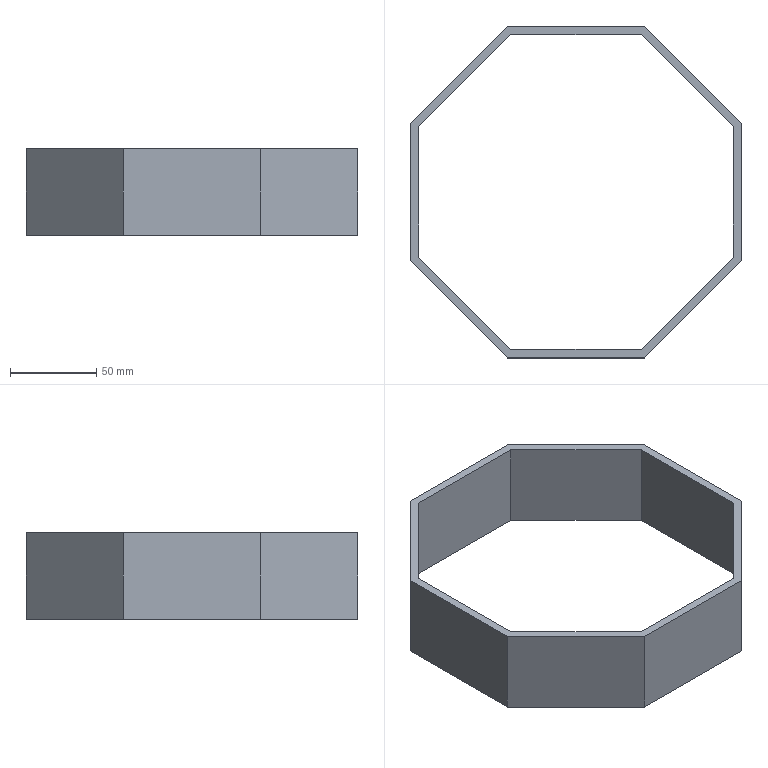Part | SolidWorks | features Extrusion 1, ICE 1 | 1 solid | 18 faces | box 192.167 x 192.167 x 50 mm | volume 155054 mm3 | plane 18
STEP:
#1=CARTESIAN_POINT('',(39.799,96.083,0.));
#2=VERTEX_POINT('',#1);
#3=CARTESIAN_POINT('',(-39.799,96.083,0.));
#4=VERTEX_POINT('',#3);
#5=CARTESIAN_POINT('',(39.799,96.083,0.));
#6=DIRECTION('',(-1.,0.,0.));
#7=VECTOR('',#6,1000.);
#8=LINE('',#5,#7);
#9=EDGE_CURVE('',#2,#4,#8,.T.);
#10=ORIENTED_EDGE('',*,*,#9,.T.);
#11=CARTESIAN_POINT('',(-39.799,96.083,50.));
#12=VERTEX_POINT('',#11);
#13=CARTESIAN_POINT('',(-39.799,96.083,50.));
#14=DIRECTION('',(0.,0.,-1.));
#15=VECTOR('',#14,1000.);
#16=LINE('',#13,#15);
#17=EDGE_CURVE('',#12,#4,#16,.T.);
#18=ORIENTED_EDGE('',*,*,#17,.F.);
#19=CARTESIAN_POINT('',(39.799,96.083,50.));
#20=VERTEX_POINT('',#19);
#21=CARTESIAN_POINT('',(39.799,96.083,50.));
#22=DIRECTION('',(-1.,0.,0.));
#23=VECTOR('',#22,1000.);
#24=LINE('',#21,#23);
#25=EDGE_CURVE('',#20,#12,#24,.T.);
#26=ORIENTED_EDGE('',*,*,#25,.F.);
#27=CARTESIAN_POINT('',(39.799,96.083,50.));
#28=DIRECTION('',(0.,0.,-1.));
#29=VECTOR('',#28,1000.);
#30=LINE('',#27,#29);
#31=EDGE_CURVE('',#20,#2,#30,.T.);
#32=ORIENTED_EDGE('',*,*,#31,.T.);
#33=EDGE_LOOP('',(#10,#18,#26,#32));
#34=FACE_OUTER_BOUND('',#33,.T.);
#35=CARTESIAN_POINT('',(39.799,96.083,50.));
#36=DIRECTION('',(0.,-1.,0.));
#37=DIRECTION('',(0.,0.,-1.));
#38=AXIS2_PLACEMENT_3D('',#35,#36,#37);
#39=PLANE('',#38);
#40=ADVANCED_FACE('',(#34),#39,.F.);
#41=CARTESIAN_POINT('',(-96.083,39.799,0.));
#42=VERTEX_POINT('',#41);
#43=CARTESIAN_POINT('',(-39.799,96.083,0.));
#44=DIRECTION('',(-0.7071,-0.7071,0.));
#45=VECTOR('',#44,1000.);
#46=LINE('',#43,#45);
#47=EDGE_CURVE('',#4,#42,#46,.T.);
#48=ORIENTED_EDGE('',*,*,#47,.T.);
#49=CARTESIAN_POINT('',(-96.083,39.799,50.));
#50=VERTEX_POINT('',#49);
#51=CARTESIAN_POINT('',(-96.083,39.799,50.));
#52=DIRECTION('',(0.,0.,-1.));
#53=VECTOR('',#52,1000.);
#54=LINE('',#51,#53);
#55=EDGE_CURVE('',#50,#42,#54,.T.);
#56=ORIENTED_EDGE('',*,*,#55,.F.);
#57=CARTESIAN_POINT('',(-39.799,96.083,50.));
#58=DIRECTION('',(-0.7071,-0.7071,0.));
#59=VECTOR('',#58,1000.);
#60=LINE('',#57,#59);
#61=EDGE_CURVE('',#12,#50,#60,.T.);
#62=ORIENTED_EDGE('',*,*,#61,.F.);
#63=ORIENTED_EDGE('',*,*,#17,.T.);
#64=EDGE_LOOP('',(#48,#56,#62,#63));
#65=FACE_OUTER_BOUND('',#64,.T.);
#66=CARTESIAN_POINT('',(-39.799,96.083,50.));
#67=DIRECTION('',(0.7071,-0.7071,0.));
#68=DIRECTION('',(0.7071,0.7071,0.));
#69=AXIS2_PLACEMENT_3D('',#66,#67,#68);
#70=PLANE('',#69);
#71=ADVANCED_FACE('',(#65),#70,.F.);
#72=CARTESIAN_POINT('',(-96.083,-39.799,0.));
#73=VERTEX_POINT('',#72);
#74=CARTESIAN_POINT('',(-96.083,39.799,0.));
#75=DIRECTION('',(0.,-1.,0.));
#76=VECTOR('',#75,1000.);
#77=LINE('',#74,#76);
#78=EDGE_CURVE('',#42,#73,#77,.T.);
#79=ORIENTED_EDGE('',*,*,#78,.T.);
#80=CARTESIAN_POINT('',(-96.083,-39.799,50.));
#81=VERTEX_POINT('',#80);
#82=CARTESIAN_POINT('',(-96.083,-39.799,50.));
#83=DIRECTION('',(0.,0.,-1.));
#84=VECTOR('',#83,1000.);
#85=LINE('',#82,#84);
#86=EDGE_CURVE('',#81,#73,#85,.T.);
#87=ORIENTED_EDGE('',*,*,#86,.F.);
#88=CARTESIAN_POINT('',(-96.083,39.799,50.));
#89=DIRECTION('',(0.,-1.,0.));
#90=VECTOR('',#89,1000.);
#91=LINE('',#88,#90);
#92=EDGE_CURVE('',#50,#81,#91,.T.);
#93=ORIENTED_EDGE('',*,*,#92,.F.);
#94=ORIENTED_EDGE('',*,*,#55,.T.);
#95=EDGE_LOOP('',(#79,#87,#93,#94));
#96=FACE_OUTER_BOUND('',#95,.T.);
#97=CARTESIAN_POINT('',(-96.083,39.799,50.));
#98=DIRECTION('',(1.,0.,0.));
#99=DIRECTION('',(0.,1.,0.));
#100=AXIS2_PLACEMENT_3D('',#97,#98,#99);
#101=PLANE('',#100);
#102=ADVANCED_FACE('',(#96),#101,.F.);
#103=CARTESIAN_POINT('',(-39.799,-96.083,0.));
#104=VERTEX_POINT('',#103);
#105=CARTESIAN_POINT('',(-96.083,-39.799,0.));
#106=DIRECTION('',(0.7071,-0.7071,0.));
#107=VECTOR('',#106,1000.);
#108=LINE('',#105,#107);
#109=EDGE_CURVE('',#73,#104,#108,.T.);
#110=ORIENTED_EDGE('',*,*,#109,.T.);
#111=CARTESIAN_POINT('',(-39.799,-96.083,50.));
#112=VERTEX_POINT('',#111);
#113=CARTESIAN_POINT('',(-39.799,-96.083,50.));
#114=DIRECTION('',(0.,0.,-1.));
#115=VECTOR('',#114,1000.);
#116=LINE('',#113,#115);
#117=EDGE_CURVE('',#112,#104,#116,.T.);
#118=ORIENTED_EDGE('',*,*,#117,.F.);
#119=CARTESIAN_POINT('',(-96.083,-39.799,50.));
#120=DIRECTION('',(0.7071,-0.7071,0.));
#121=VECTOR('',#120,1000.);
#122=LINE('',#119,#121);
#123=EDGE_CURVE('',#81,#112,#122,.T.);
#124=ORIENTED_EDGE('',*,*,#123,.F.);
#125=ORIENTED_EDGE('',*,*,#86,.T.);
#126=EDGE_LOOP('',(#110,#118,#124,#125));
#127=FACE_OUTER_BOUND('',#126,.T.);
#128=CARTESIAN_POINT('',(-96.083,-39.799,50.));
#129=DIRECTION('',(0.7071,0.7071,0.));
#130=DIRECTION('',(-0.7071,0.7071,0.));
#131=AXIS2_PLACEMENT_3D('',#128,#129,#130);
#132=PLANE('',#131);
#133=ADVANCED_FACE('',(#127),#132,.F.);
#134=CARTESIAN_POINT('',(39.799,-96.083,0.));
#135=VERTEX_POINT('',#134);
#136=CARTESIAN_POINT('',(-39.799,-96.083,0.));
#137=DIRECTION('',(1.,0.,0.));
#138=VECTOR('',#137,1000.);
#139=LINE('',#136,#138);
#140=EDGE_CURVE('',#104,#135,#139,.T.);
#141=ORIENTED_EDGE('',*,*,#140,.T.);
#142=CARTESIAN_POINT('',(39.799,-96.083,50.));
#143=VERTEX_POINT('',#142);
#144=CARTESIAN_POINT('',(39.799,-96.083,50.));
#145=DIRECTION('',(0.,0.,-1.));
#146=VECTOR('',#145,1000.);
#147=LINE('',#144,#146);
#148=EDGE_CURVE('',#143,#135,#147,.T.);
#149=ORIENTED_EDGE('',*,*,#148,.F.);
#150=CARTESIAN_POINT('',(-39.799,-96.083,50.));
#151=DIRECTION('',(1.,0.,0.));
#152=VECTOR('',#151,1000.);
#153=LINE('',#150,#152);
#154=EDGE_CURVE('',#112,#143,#153,.T.);
#155=ORIENTED_EDGE('',*,*,#154,.F.);
#156=ORIENTED_EDGE('',*,*,#117,.T.);
#157=EDGE_LOOP('',(#141,#149,#155,#156));
#158=FACE_OUTER_BOUND('',#157,.T.);
#159=CARTESIAN_POINT('',(-39.799,-96.083,50.));
#160=DIRECTION('',(0.,1.,0.));
#161=DIRECTION('',(-1.,0.,0.));
#162=AXIS2_PLACEMENT_3D('',#159,#160,#161);
#163=PLANE('',#162);
#164=ADVANCED_FACE('',(#158),#163,.F.);
#165=CARTESIAN_POINT('',(96.083,-39.799,0.));
#166=VERTEX_POINT('',#165);
#167=CARTESIAN_POINT('',(39.799,-96.083,0.));
#168=DIRECTION('',(0.7071,0.7071,0.));
#169=VECTOR('',#168,1000.);
#170=LINE('',#167,#169);
#171=EDGE_CURVE('',#135,#166,#170,.T.);
#172=ORIENTED_EDGE('',*,*,#171,.T.);
#173=CARTESIAN_POINT('',(96.083,-39.799,50.));
#174=VERTEX_POINT('',#173);
#175=CARTESIAN_POINT('',(96.083,-39.799,50.));
#176=DIRECTION('',(0.,0.,-1.));
#177=VECTOR('',#176,1000.);
#178=LINE('',#175,#177);
#179=EDGE_CURVE('',#174,#166,#178,.T.);
#180=ORIENTED_EDGE('',*,*,#179,.F.);
#181=CARTESIAN_POINT('',(39.799,-96.083,50.));
#182=DIRECTION('',(0.7071,0.7071,0.));
#183=VECTOR('',#182,1000.);
#184=LINE('',#181,#183);
#185=EDGE_CURVE('',#143,#174,#184,.T.);
#186=ORIENTED_EDGE('',*,*,#185,.F.);
#187=ORIENTED_EDGE('',*,*,#148,.T.);
#188=EDGE_LOOP('',(#172,#180,#186,#187));
#189=FACE_OUTER_BOUND('',#188,.T.);
#190=CARTESIAN_POINT('',(39.799,-96.083,50.));
#191=DIRECTION('',(-0.7071,0.7071,0.));
#192=DIRECTION('',(-0.7071,-0.7071,0.));
#193=AXIS2_PLACEMENT_3D('',#190,#191,#192);
#194=PLANE('',#193);
#195=ADVANCED_FACE('',(#189),#194,.F.);
#196=CARTESIAN_POINT('',(96.083,39.799,0.));
#197=VERTEX_POINT('',#196);
#198=CARTESIAN_POINT('',(96.083,-39.799,0.));
#199=DIRECTION('',(0.,1.,0.));
#200=VECTOR('',#199,1000.);
#201=LINE('',#198,#200);
#202=EDGE_CURVE('',#166,#197,#201,.T.);
#203=ORIENTED_EDGE('',*,*,#202,.T.);
#204=CARTESIAN_POINT('',(96.083,39.799,50.));
#205=VERTEX_POINT('',#204);
#206=CARTESIAN_POINT('',(96.083,39.799,50.));
#207=DIRECTION('',(0.,0.,-1.));
#208=VECTOR('',#207,1000.);
#209=LINE('',#206,#208);
#210=EDGE_CURVE('',#205,#197,#209,.T.);
#211=ORIENTED_EDGE('',*,*,#210,.F.);
#212=CARTESIAN_POINT('',(96.083,-39.799,50.));
#213=DIRECTION('',(0.,1.,0.));
#214=VECTOR('',#213,1000.);
#215=LINE('',#212,#214);
#216=EDGE_CURVE('',#174,#205,#215,.T.);
#217=ORIENTED_EDGE('',*,*,#216,.F.);
#218=ORIENTED_EDGE('',*,*,#179,.T.);
#219=EDGE_LOOP('',(#203,#211,#217,#218));
#220=FACE_OUTER_BOUND('',#219,.T.);
#221=CARTESIAN_POINT('',(96.083,-39.799,50.));
#222=DIRECTION('',(-1.,0.,0.));
#223=DIRECTION('',(0.,0.,1.));
#224=AXIS2_PLACEMENT_3D('',#221,#222,#223);
#225=PLANE('',#224);
#226=ADVANCED_FACE('',(#220),#225,.F.);
#227=CARTESIAN_POINT('',(96.083,39.799,0.));
#228=DIRECTION('',(-0.7071,0.7071,0.));
#229=VECTOR('',#228,1000.);
#230=LINE('',#227,#229);
#231=EDGE_CURVE('',#197,#2,#230,.T.);
#232=ORIENTED_EDGE('',*,*,#231,.T.);
#233=ORIENTED_EDGE('',*,*,#31,.F.);
#234=CARTESIAN_POINT('',(96.083,39.799,50.));
#235=DIRECTION('',(-0.7071,0.7071,0.));
#236=VECTOR('',#235,1000.);
#237=LINE('',#234,#236);
#238=EDGE_CURVE('',#205,#20,#237,.T.);
#239=ORIENTED_EDGE('',*,*,#238,.F.);
#240=ORIENTED_EDGE('',*,*,#210,.T.);
#241=EDGE_LOOP('',(#232,#233,#239,#240));
#242=FACE_OUTER_BOUND('',#241,.T.);
#243=CARTESIAN_POINT('',(96.083,39.799,50.));
#244=DIRECTION('',(-0.7071,-0.7071,0.));
#245=DIRECTION('',(0.7071,-0.7071,0.));
#246=AXIS2_PLACEMENT_3D('',#243,#244,#245);
#247=PLANE('',#246);
#248=ADVANCED_FACE('',(#242),#247,.F.);
#249=CARTESIAN_POINT('',(91.083,37.728,50.));
#250=VERTEX_POINT('',#249);
#251=CARTESIAN_POINT('',(37.728,91.083,50.));
#252=VERTEX_POINT('',#251);
#253=CARTESIAN_POINT('',(91.083,37.728,50.));
#254=DIRECTION('',(-0.7071,0.7071,0.));
#255=VECTOR('',#254,1000.);
#256=LINE('',#253,#255);
#257=EDGE_CURVE('',#250,#252,#256,.T.);
#258=ORIENTED_EDGE('',*,*,#257,.F.);
#259=CARTESIAN_POINT('',(91.083,-37.728,50.));
#260=VERTEX_POINT('',#259);
#261=CARTESIAN_POINT('',(91.083,-37.728,50.));
#262=DIRECTION('',(0.,1.,0.));
#263=VECTOR('',#262,1000.);
#264=LINE('',#261,#263);
#265=EDGE_CURVE('',#260,#250,#264,.T.);
#266=ORIENTED_EDGE('',*,*,#265,.F.);
#267=CARTESIAN_POINT('',(37.728,-91.083,50.));
#268=VERTEX_POINT('',#267);
#269=CARTESIAN_POINT('',(37.728,-91.083,50.));
#270=DIRECTION('',(0.7071,0.7071,0.));
#271=VECTOR('',#270,1000.);
#272=LINE('',#269,#271);
#273=EDGE_CURVE('',#268,#260,#272,.T.);
#274=ORIENTED_EDGE('',*,*,#273,.F.);
#275=CARTESIAN_POINT('',(-37.728,-91.083,50.));
#276=VERTEX_POINT('',#275);
#277=CARTESIAN_POINT('',(-37.728,-91.083,50.));
#278=DIRECTION('',(1.,0.,0.));
#279=VECTOR('',#278,1000.);
#280=LINE('',#277,#279);
#281=EDGE_CURVE('',#276,#268,#280,.T.);
#282=ORIENTED_EDGE('',*,*,#281,.F.);
#283=CARTESIAN_POINT('',(-91.083,-37.728,50.));
#284=VERTEX_POINT('',#283);
#285=CARTESIAN_POINT('',(-91.083,-37.728,50.));
#286=DIRECTION('',(0.7071,-0.7071,0.));
#287=VECTOR('',#286,1000.);
#288=LINE('',#285,#287);
#289=EDGE_CURVE('',#284,#276,#288,.T.);
#290=ORIENTED_EDGE('',*,*,#289,.F.);
#291=CARTESIAN_POINT('',(-91.083,37.728,50.));
#292=VERTEX_POINT('',#291);
#293=CARTESIAN_POINT('',(-91.083,37.728,50.));
#294=DIRECTION('',(0.,-1.,0.));
#295=VECTOR('',#294,1000.);
#296=LINE('',#293,#295);
#297=EDGE_CURVE('',#292,#284,#296,.T.);
#298=ORIENTED_EDGE('',*,*,#297,.F.);
#299=CARTESIAN_POINT('',(-37.728,91.083,50.));
#300=VERTEX_POINT('',#299);
#301=CARTESIAN_POINT('',(-37.728,91.083,50.));
#302=DIRECTION('',(-0.7071,-0.7071,0.));
#303=VECTOR('',#302,1000.);
#304=LINE('',#301,#303);
#305=EDGE_CURVE('',#300,#292,#304,.T.);
#306=ORIENTED_EDGE('',*,*,#305,.F.);
#307=CARTESIAN_POINT('',(37.728,91.083,50.));
#308=DIRECTION('',(-1.,0.,0.));
#309=VECTOR('',#308,1000.);
#310=LINE('',#307,#309);
#311=EDGE_CURVE('',#252,#300,#310,.T.);
#312=ORIENTED_EDGE('',*,*,#311,.F.);
#313=EDGE_LOOP('',(#258,#266,#274,#282,#290,#298,#306,#312));
#314=FACE_BOUND('',#313,.T.);
#315=ORIENTED_EDGE('',*,*,#25,.T.);
#316=ORIENTED_EDGE('',*,*,#61,.T.);
#317=ORIENTED_EDGE('',*,*,#92,.T.);
#318=ORIENTED_EDGE('',*,*,#123,.T.);
#319=ORIENTED_EDGE('',*,*,#154,.T.);
#320=ORIENTED_EDGE('',*,*,#185,.T.);
#321=ORIENTED_EDGE('',*,*,#216,.T.);
#322=ORIENTED_EDGE('',*,*,#238,.T.);
#323=EDGE_LOOP('',(#315,#316,#317,#318,#319,#320,#321,#322));
#324=FACE_OUTER_BOUND('',#323,.T.);
#325=CARTESIAN_POINT('',(0.,0.,50.));
#326=DIRECTION('',(0.,0.,1.));
#327=DIRECTION('',(1.,0.,0.));
#328=AXIS2_PLACEMENT_3D('',#325,#326,#327);
#329=PLANE('',#328);
#330=ADVANCED_FACE('',(#314,#324),#329,.T.);
#331=CARTESIAN_POINT('',(91.083,-37.728,0.));
#332=VERTEX_POINT('',#331);
#333=CARTESIAN_POINT('',(91.083,37.728,0.));
#334=VERTEX_POINT('',#333);
#335=CARTESIAN_POINT('',(91.083,0.,0.));
#336=DIRECTION('',(0.,1.,0.));
#337=VECTOR('',#336,1000.);
#338=LINE('',#335,#337);
#339=EDGE_CURVE('',#332,#334,#338,.T.);
#340=ORIENTED_EDGE('',*,*,#339,.T.);
#341=CARTESIAN_POINT('',(37.728,91.083,0.));
#342=VERTEX_POINT('',#341);
#343=CARTESIAN_POINT('',(64.406,64.406,0.));
#344=DIRECTION('',(-0.7071,0.7071,0.));
#345=VECTOR('',#344,1000.);
#346=LINE('',#343,#345);
#347=EDGE_CURVE('',#334,#342,#346,.T.);
#348=ORIENTED_EDGE('',*,*,#347,.T.);
#349=CARTESIAN_POINT('',(-37.728,91.083,0.));
#350=VERTEX_POINT('',#349);
#351=CARTESIAN_POINT('',(0.,91.083,0.));
#352=DIRECTION('',(-1.,0.,0.));
#353=VECTOR('',#352,1000.);
#354=LINE('',#351,#353);
#355=EDGE_CURVE('',#342,#350,#354,.T.);
#356=ORIENTED_EDGE('',*,*,#355,.T.);
#357=CARTESIAN_POINT('',(-91.083,37.728,0.));
#358=VERTEX_POINT('',#357);
#359=CARTESIAN_POINT('',(-64.406,64.406,0.));
#360=DIRECTION('',(-0.7071,-0.7071,0.));
#361=VECTOR('',#360,1000.);
#362=LINE('',#359,#361);
#363=EDGE_CURVE('',#350,#358,#362,.T.);
#364=ORIENTED_EDGE('',*,*,#363,.T.);
#365=CARTESIAN_POINT('',(-91.083,-37.728,0.));
#366=VERTEX_POINT('',#365);
#367=CARTESIAN_POINT('',(-91.083,0.,0.));
#368=DIRECTION('',(0.,-1.,0.));
#369=VECTOR('',#368,1000.);
#370=LINE('',#367,#369);
#371=EDGE_CURVE('',#358,#366,#370,.T.);
#372=ORIENTED_EDGE('',*,*,#371,.T.);
#373=CARTESIAN_POINT('',(-37.728,-91.083,0.));
#374=VERTEX_POINT('',#373);
#375=CARTESIAN_POINT('',(-64.406,-64.406,0.));
#376=DIRECTION('',(0.7071,-0.7071,0.));
#377=VECTOR('',#376,1000.);
#378=LINE('',#375,#377);
#379=EDGE_CURVE('',#366,#374,#378,.T.);
#380=ORIENTED_EDGE('',*,*,#379,.T.);
#381=CARTESIAN_POINT('',(37.728,-91.083,0.));
#382=VERTEX_POINT('',#381);
#383=CARTESIAN_POINT('',(0.,-91.083,0.));
#384=DIRECTION('',(1.,0.,0.));
#385=VECTOR('',#384,1000.);
#386=LINE('',#383,#385);
#387=EDGE_CURVE('',#374,#382,#386,.T.);
#388=ORIENTED_EDGE('',*,*,#387,.T.);
#389=CARTESIAN_POINT('',(64.406,-64.406,0.));
#390=DIRECTION('',(0.7071,0.7071,0.));
#391=VECTOR('',#390,1000.);
#392=LINE('',#389,#391);
#393=EDGE_CURVE('',#382,#332,#392,.T.);
#394=ORIENTED_EDGE('',*,*,#393,.T.);
#395=EDGE_LOOP('',(#340,#348,#356,#364,#372,#380,#388,#394));
#396=FACE_BOUND('',#395,.T.);
#397=ORIENTED_EDGE('',*,*,#9,.F.);
#398=ORIENTED_EDGE('',*,*,#231,.F.);
#399=ORIENTED_EDGE('',*,*,#202,.F.);
#400=ORIENTED_EDGE('',*,*,#171,.F.);
#401=ORIENTED_EDGE('',*,*,#140,.F.);
#402=ORIENTED_EDGE('',*,*,#109,.F.);
#403=ORIENTED_EDGE('',*,*,#78,.F.);
#404=ORIENTED_EDGE('',*,*,#47,.F.);
#405=EDGE_LOOP('',(#397,#398,#399,#400,#401,#402,#403,#404));
#406=FACE_OUTER_BOUND('',#405,.T.);
#407=CARTESIAN_POINT('',(0.,0.,0.));
#408=DIRECTION('',(0.,0.,1.));
#409=DIRECTION('',(1.,0.,0.));
#410=AXIS2_PLACEMENT_3D('',#407,#408,#409);
#411=PLANE('',#410);
#412=ADVANCED_FACE('',(#396,#406),#411,.F.);
#413=CARTESIAN_POINT('',(91.083,37.728,-556.));
#414=DIRECTION('',(0.,0.,1.));
#415=VECTOR('',#414,1000.);
#416=LINE('',#413,#415);
#417=EDGE_CURVE('',#334,#250,#416,.T.);
#418=ORIENTED_EDGE('',*,*,#417,.T.);
#419=ORIENTED_EDGE('',*,*,#257,.T.);
#420=CARTESIAN_POINT('',(37.728,91.083,-556.));
#421=DIRECTION('',(0.,0.,1.));
#422=VECTOR('',#421,1000.);
#423=LINE('',#420,#422);
#424=EDGE_CURVE('',#342,#252,#423,.T.);
#425=ORIENTED_EDGE('',*,*,#424,.F.);
#426=ORIENTED_EDGE('',*,*,#347,.F.);
#427=EDGE_LOOP('',(#418,#419,#425,#426));
#428=FACE_OUTER_BOUND('',#427,.T.);
#429=CARTESIAN_POINT('',(91.083,37.728,-556.));
#430=DIRECTION('',(0.7071,0.7071,0.));
#431=DIRECTION('',(-0.7071,0.7071,0.));
#432=AXIS2_PLACEMENT_3D('',#429,#430,#431);
#433=PLANE('',#432);
#434=ADVANCED_FACE('',(#428),#433,.F.);
#435=CARTESIAN_POINT('',(91.083,-37.728,-556.));
#436=DIRECTION('',(0.,0.,1.));
#437=VECTOR('',#436,1000.);
#438=LINE('',#435,#437);
#439=EDGE_CURVE('',#332,#260,#438,.T.);
#440=ORIENTED_EDGE('',*,*,#439,.T.);
#441=ORIENTED_EDGE('',*,*,#265,.T.);
#442=ORIENTED_EDGE('',*,*,#417,.F.);
#443=ORIENTED_EDGE('',*,*,#339,.F.);
#444=EDGE_LOOP('',(#440,#441,#442,#443));
#445=FACE_OUTER_BOUND('',#444,.T.);
#446=CARTESIAN_POINT('',(91.083,-37.728,-556.));
#447=DIRECTION('',(1.,0.,0.));
#448=DIRECTION('',(0.,0.,-1.));
#449=AXIS2_PLACEMENT_3D('',#446,#447,#448);
#450=PLANE('',#449);
#451=ADVANCED_FACE('',(#445),#450,.F.);
#452=CARTESIAN_POINT('',(37.728,-91.083,-556.));
#453=DIRECTION('',(0.,0.,1.));
#454=VECTOR('',#453,1000.);
#455=LINE('',#452,#454);
#456=EDGE_CURVE('',#382,#268,#455,.T.);
#457=ORIENTED_EDGE('',*,*,#456,.T.);
#458=ORIENTED_EDGE('',*,*,#273,.T.);
#459=ORIENTED_EDGE('',*,*,#439,.F.);
#460=ORIENTED_EDGE('',*,*,#393,.F.);
#461=EDGE_LOOP('',(#457,#458,#459,#460));
#462=FACE_OUTER_BOUND('',#461,.T.);
#463=CARTESIAN_POINT('',(37.728,-91.083,-556.));
#464=DIRECTION('',(0.7071,-0.7071,0.));
#465=DIRECTION('',(0.7071,0.7071,0.));
#466=AXIS2_PLACEMENT_3D('',#463,#464,#465);
#467=PLANE('',#466);
#468=ADVANCED_FACE('',(#462),#467,.F.);
#469=CARTESIAN_POINT('',(-37.728,-91.083,-556.));
#470=DIRECTION('',(0.,0.,1.));
#471=VECTOR('',#470,1000.);
#472=LINE('',#469,#471);
#473=EDGE_CURVE('',#374,#276,#472,.T.);
#474=ORIENTED_EDGE('',*,*,#473,.T.);
#475=ORIENTED_EDGE('',*,*,#281,.T.);
#476=ORIENTED_EDGE('',*,*,#456,.F.);
#477=ORIENTED_EDGE('',*,*,#387,.F.);
#478=EDGE_LOOP('',(#474,#475,#476,#477));
#479=FACE_OUTER_BOUND('',#478,.T.);
#480=CARTESIAN_POINT('',(-37.728,-91.083,-556.));
#481=DIRECTION('',(0.,-1.,0.));
#482=DIRECTION('',(1.,0.,0.));
#483=AXIS2_PLACEMENT_3D('',#480,#481,#482);
#484=PLANE('',#483);
#485=ADVANCED_FACE('',(#479),#484,.F.);
#486=CARTESIAN_POINT('',(-91.083,-37.728,-556.));
#487=DIRECTION('',(0.,0.,1.));
#488=VECTOR('',#487,1000.);
#489=LINE('',#486,#488);
#490=EDGE_CURVE('',#366,#284,#489,.T.);
#491=ORIENTED_EDGE('',*,*,#490,.T.);
#492=ORIENTED_EDGE('',*,*,#289,.T.);
#493=ORIENTED_EDGE('',*,*,#473,.F.);
#494=ORIENTED_EDGE('',*,*,#379,.F.);
#495=EDGE_LOOP('',(#491,#492,#493,#494));
#496=FACE_OUTER_BOUND('',#495,.T.);
#497=CARTESIAN_POINT('',(-91.083,-37.728,-556.));
#498=DIRECTION('',(-0.7071,-0.7071,0.));
#499=DIRECTION('',(0.7071,-0.7071,0.));
#500=AXIS2_PLACEMENT_3D('',#497,#498,#499);
#501=PLANE('',#500);
#502=ADVANCED_FACE('',(#496),#501,.F.);
#503=CARTESIAN_POINT('',(-91.083,37.728,-556.));
#504=DIRECTION('',(0.,0.,1.));
#505=VECTOR('',#504,1000.);
#506=LINE('',#503,#505);
#507=EDGE_CURVE('',#358,#292,#506,.T.);
#508=ORIENTED_EDGE('',*,*,#507,.T.);
#509=ORIENTED_EDGE('',*,*,#297,.T.);
#510=ORIENTED_EDGE('',*,*,#490,.F.);
#511=ORIENTED_EDGE('',*,*,#371,.F.);
#512=EDGE_LOOP('',(#508,#509,#510,#511));
#513=FACE_OUTER_BOUND('',#512,.T.);
#514=CARTESIAN_POINT('',(-91.083,37.728,-556.));
#515=DIRECTION('',(-1.,0.,0.));
#516=DIRECTION('',(0.,-1.,0.));
#517=AXIS2_PLACEMENT_3D('',#514,#515,#516);
#518=PLANE('',#517);
#519=ADVANCED_FACE('',(#513),#518,.F.);
#520=CARTESIAN_POINT('',(-37.728,91.083,-556.));
#521=DIRECTION('',(0.,0.,1.));
#522=VECTOR('',#521,1000.);
#523=LINE('',#520,#522);
#524=EDGE_CURVE('',#350,#300,#523,.T.);
#525=ORIENTED_EDGE('',*,*,#524,.T.);
#526=ORIENTED_EDGE('',*,*,#305,.T.);
#527=ORIENTED_EDGE('',*,*,#507,.F.);
#528=ORIENTED_EDGE('',*,*,#363,.F.);
#529=EDGE_LOOP('',(#525,#526,#527,#528));
#530=FACE_OUTER_BOUND('',#529,.T.);
#531=CARTESIAN_POINT('',(-37.728,91.083,-556.));
#532=DIRECTION('',(-0.7071,0.7071,0.));
#533=DIRECTION('',(-0.7071,-0.7071,0.));
#534=AXIS2_PLACEMENT_3D('',#531,#532,#533);
#535=PLANE('',#534);
#536=ADVANCED_FACE('',(#530),#535,.F.);
#537=ORIENTED_EDGE('',*,*,#424,.T.);
#538=ORIENTED_EDGE('',*,*,#311,.T.);
#539=ORIENTED_EDGE('',*,*,#524,.F.);
#540=ORIENTED_EDGE('',*,*,#355,.F.);
#541=EDGE_LOOP('',(#537,#538,#539,#540));
#542=FACE_OUTER_BOUND('',#541,.T.);
#543=CARTESIAN_POINT('',(37.728,91.083,-556.));
#544=DIRECTION('',(0.,1.,0.));
#545=DIRECTION('',(0.,0.,1.));
#546=AXIS2_PLACEMENT_3D('',#543,#544,#545);
#547=PLANE('',#546);
#548=ADVANCED_FACE('',(#542),#547,.F.);
#549=CLOSED_SHELL('',(#40,#71,#102,#133,#164,#195,#226,#248,#330,#412,#434,#451,#468,#485,#502,#519,#536,#548));
#550=MANIFOLD_SOLID_BREP('',#549);
#551=CARTESIAN_POINT('',(0.,0.,0.));
#552=DIRECTION('',(0.,0.,1.));
#553=DIRECTION('',(1.,0.,0.));
#554=AXIS2_PLACEMENT_3D('',#551,#552,#553);
#555=(LENGTH_UNIT()NAMED_UNIT(*)SI_UNIT(.MILLI.,.METRE.));
#556=UNCERTAINTY_MEASURE_WITH_UNIT(LENGTH_MEASURE(0.00001),#555,'','');
#557=(NAMED_UNIT(*)PLANE_ANGLE_UNIT()SI_UNIT($,.RADIAN.));
#558=(NAMED_UNIT(*)SI_UNIT($,.STERADIAN.)SOLID_ANGLE_UNIT());
#559=(GEOMETRIC_REPRESENTATION_CONTEXT(3)GLOBAL_UNCERTAINTY_ASSIGNED_CONTEXT((#556))GLOBAL_UNIT_ASSIGNED_CONTEXT((#555,#557,#558))REPRESENTATION_CONTEXT('',''));
#560=ADVANCED_BREP_SHAPE_REPRESENTATION('',(#550,#554),#559);